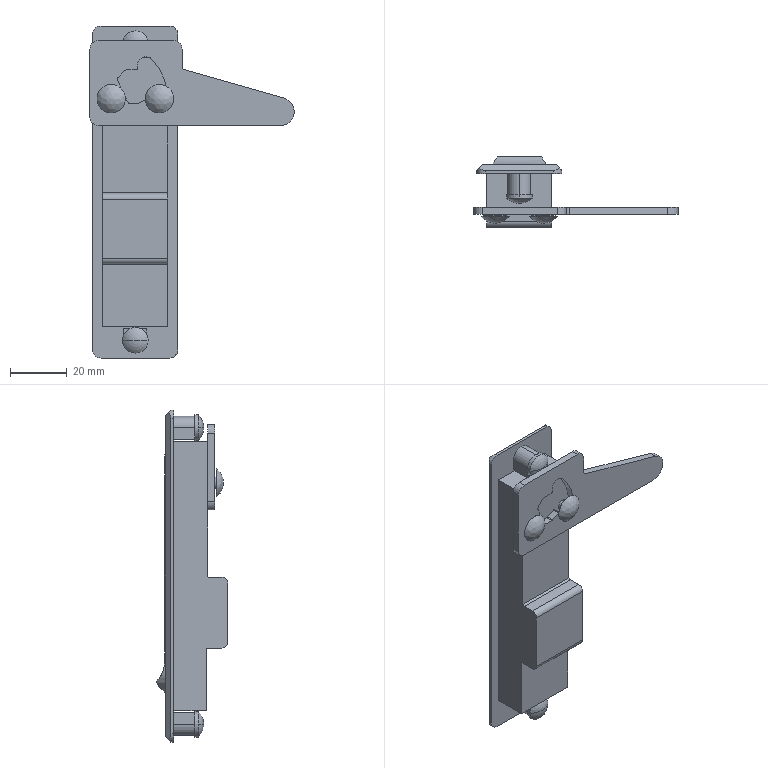Part | SolidWorks | features BaseBody 1 | 1 solid | 133 faces | box 71.998 x 25.1 x 117 mm | volume 44510 mm3 | plane 70 | cylinder 57 | torus 4 | spline 2 | commonest cylinder face diameters 6 x10 1 x9 4 x7 10 x5 9 x4 2 x3